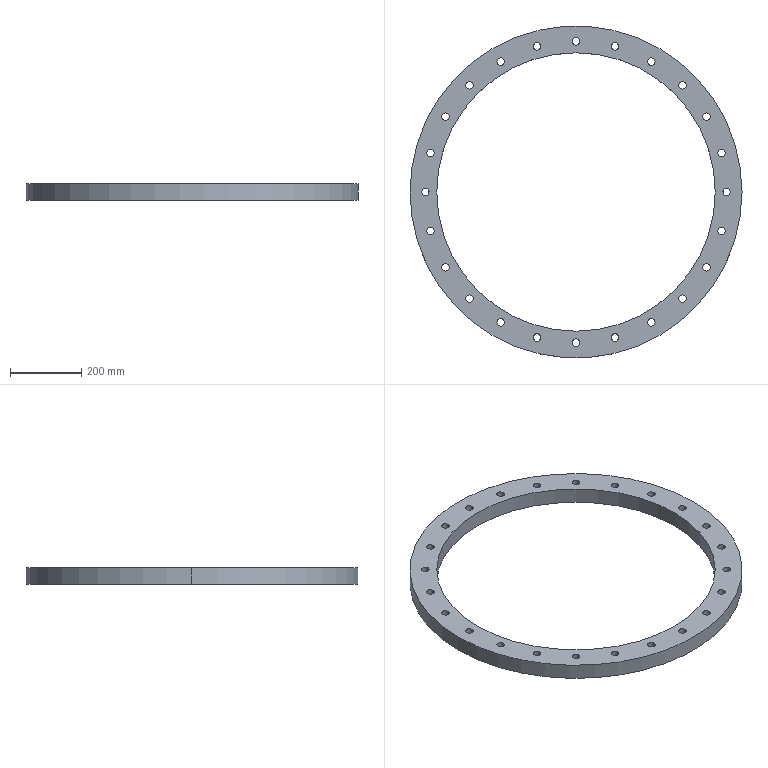Part | SolidWorks | features 3DProfileFeature 1, CirPattern 1, Extrusion 1, HoleWzd 1 | 1 solid | 54 faces | box 930 x 930 x 45 mm | volume 8691389 mm3 | cylinder 52 | plane 2 | commonest cylinder face diameters 21 x48 780 x2 930 x2